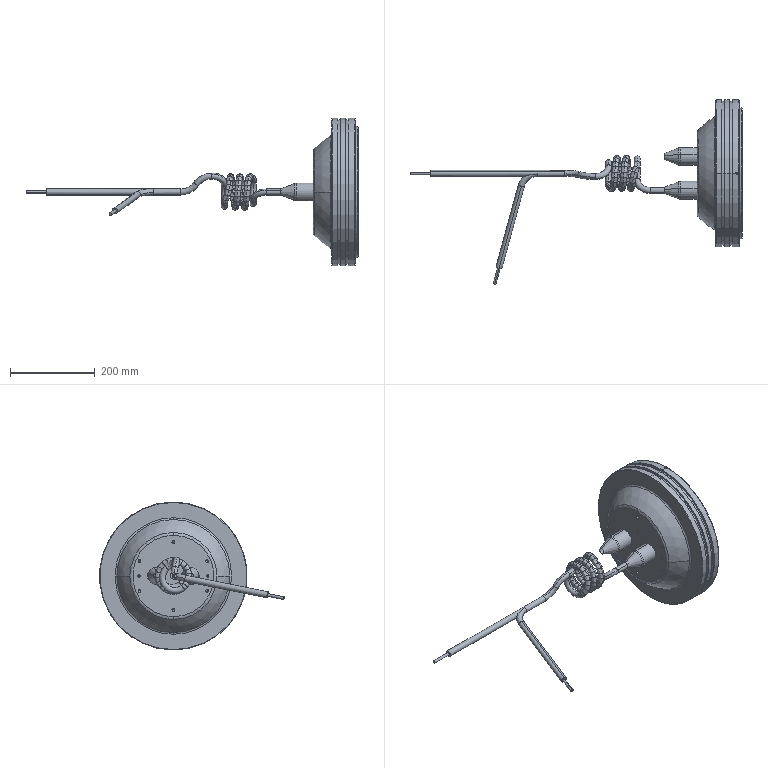Part | NX | features BREP 4 | 5 solids | 840 faces | box 785.189 x 437.108 x 350 mm | volume 7409612 mm3 | spline 279 | cylinder 210 | cone 188 | plane 86 | torus 75 | sphere 2 | commonest cylinder face diameters 30 x52 26 x48 6.8 x18 4.2 x16 6.35 x8 8.5 x8